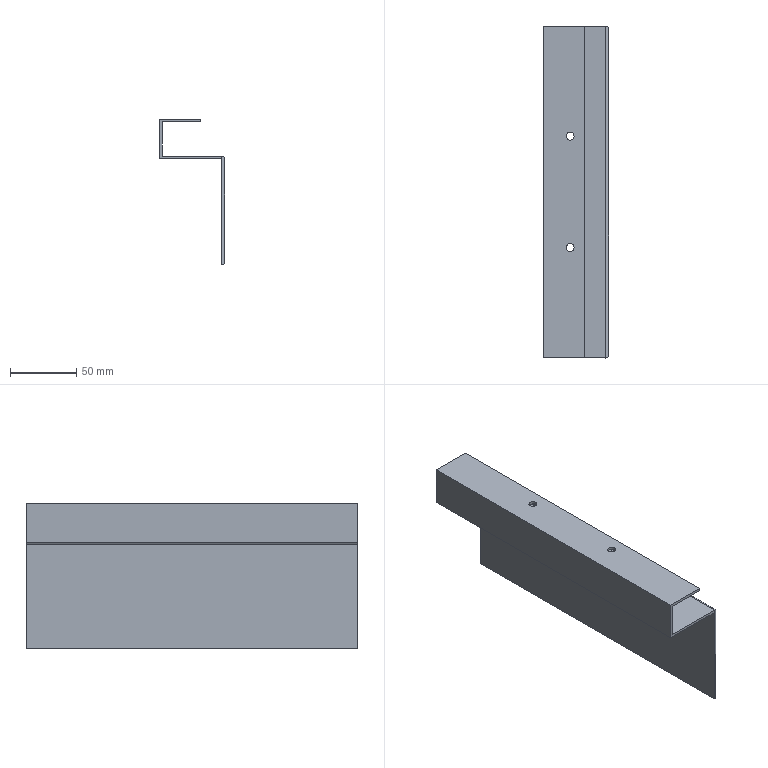Part | STEP file | zhexiayeban | 1 solid | 20 faces | box 49 x 250 x 110 mm | volume 92261 mm3 | plane 11 | cylinder 9 | commonest cylinder face diameters 4 x4 6 x4 2 x1